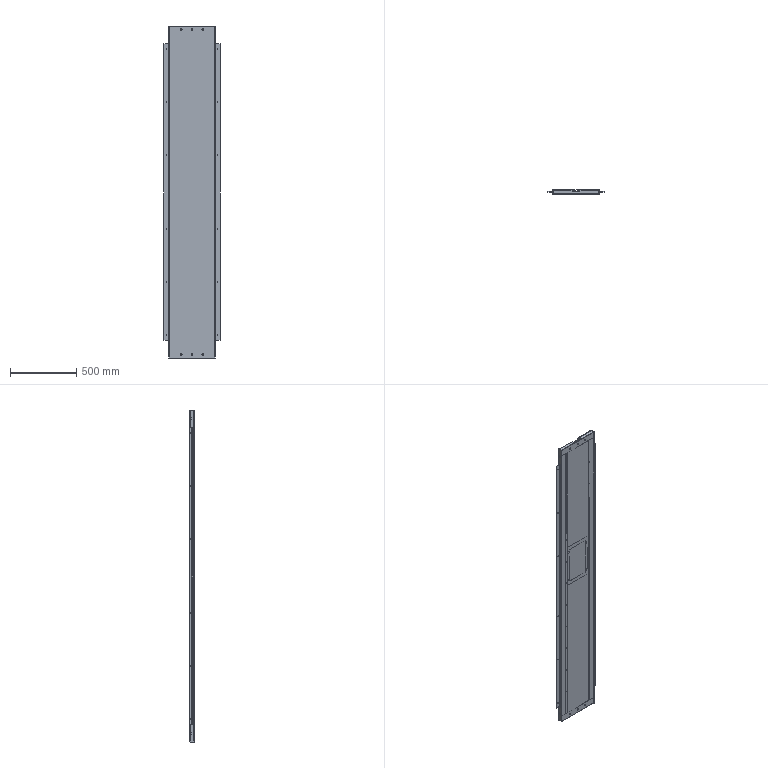Part | SolidWorks | 18 solids | 854 faces | box 424 x 33 x 2502 mm | volume 3632859 mm3 | cylinder 430 | plane 424 | commonest cylinder face diameters 6.2 x76 7 x76 5 x70 6 x44 4.5 x36 10.5 x36